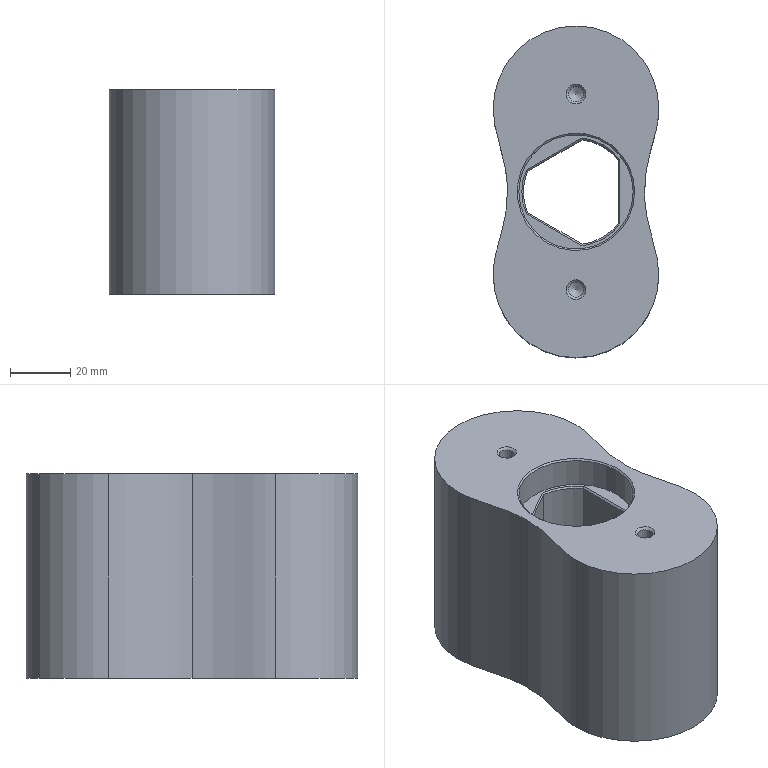NC program | NX | posted with a generic post | part box 55.004 x 110.159 x 68 mm
Lines 28 to 988 of 2889:
(ZLEVEL_PROFILE_COPY_1_COPY , TOOL : D12)
N48 M6
N50 G54
N52 G17 G0 G90 X-3.746 Y8.088 S3000 M3
N54 G43 Z30. H12
N56 Z-2.
N58 G94 G1 X-8.298 Z-2.119 F1000.
N60 X-8.881 Y7.49 Z-2.141
N62 X-10.061 Y5.809 Z-2.195
N64 X-10.927 Y3.946 Z-2.249
N66 X-11.154 Y3.143 Z-2.27
N68 X-2.855 Y-11.231 Z-2.705
N70 X-2.046 Y-11.436 Z-2.727
N72 X0. Y-11.618 Z-2.781
N74 X2.046 Y-11.436 Z-2.835
N76 X2.855 Y-11.231 Z-2.856
N78 X11.154 Y3.143 Z-3.291
N80 X10.927 Y3.946 Z-3.313
N82 X10.061 Y5.809 Z-3.367
N84 X8.881 Y7.49 Z-3.42
N86 X8.298 Y8.088 Z-3.442
N88 X-8.298 Z-3.877
N90 X-8.881 Y7.49 Z-3.899
N92 X-10.061 Y5.809 Z-3.953
N94 X-10.927 Y3.946 Z-4.006
N96 X-11.154 Y3.143 Z-4.028
N98 X-2.855 Y-11.231 Z-4.463
N100 X-2.046 Y-11.436 Z-4.485
N102 X0. Y-11.618 Z-4.538
N104 X2.046 Y-11.436 Z-4.592
N106 X2.855 Y-11.231 Z-4.614
N108 X11.154 Y3.143 Z-5.049
N110 X10.927 Y3.946 Z-5.071
N112 X10.061 Y5.809 Z-5.124
N114 X8.881 Y7.49 Z-5.178
N116 X8.298 Y8.088 Z-5.2
N118 X-8.298 F1800.
N120 G3 X-11.154 Y3.143 R11.588
N122 G1 X-2.855 Y-11.231
N124 G3 X2.855 Y-11.231 R11.588
N126 G1 X11.154 Y3.143
N128 G3 X8.298 Y8.088 R11.588
N130 G1 X-2.75 Y7.895 Z-5.393
N132 X-3.159 Y7.888 Z-5.4
N134 X-8.214
N136 G3 X-10.938 Y3.169 R11.388
N138 G1 X-2.724 Y-11.058
N140 G3 X2.724 Y-11.058 R11.388
N142 G1 X10.938 Y3.169
N144 G3 X8.214 Y7.888 R11.388
N146 G1 X7.804 Y7.882 Z-5.407
N148 X7.395 Y7.877 Z-5.414
N150 X6.986 Y7.872 Z-5.421
N152 X6.577 Y7.868 Z-5.429
N154 X6.168 Y7.864 Z-5.436
N156 X5.759 Y7.861 Z-5.443
N158 X5.349 Y7.859 Z-5.45
N160 X4.94 Y7.856 Z-5.457
N162 X4.531 Y7.854 Z-5.464
N164 X4.122 Y7.853 Z-5.471
N166 X3.712 Y7.852 Z-5.479
N168 X3.303 Y7.851 Z-5.486
N170 X2.894 Y7.85 Z-5.493
N172 X2.485 Z-5.5
N174 X-3.244 Z-5.6
N176 X-8.197
N178 G3 X-10.897 Y3.174 R11.35
N180 G1 X-2.699 Y-11.024
N182 G3 X2.7 Y-11.024 R11.35
N184 G1 X10.897 Y3.174
N186 G3 X8.198 Y7.85 R11.35
N188 G1 X-3.26 Z-5.8
N190 X-8.197
N192 G3 X-10.897 Y3.174 R11.35
N194 G1 X-2.699 Y-11.024
N196 G3 X2.7 Y-11.024 R11.35
N198 G1 X10.897 Y3.174
N200 G3 X8.198 Y7.85 R11.35
N202 G1 X-3.26 Z-6.
N204 X-8.197
N206 G3 X-10.897 Y3.174 R11.35
N208 G1 X-2.699 Y-11.024
N210 G3 X2.7 Y-11.024 R11.35
N212 G1 X10.897 Y3.174
N214 G3 X8.198 Y7.85 R11.35
N216 G1 X-3.26 Z-6.2
N218 X-8.197
N220 G3 X-10.897 Y3.174 R11.35
N222 G1 X-2.699 Y-11.024
N224 G3 X2.7 Y-11.024 R11.35
N226 G1 X10.897 Y3.174
N228 G3 X8.198 Y7.85 R11.35
N230 G1 X-3.26 Z-6.4
N232 X-8.197
N234 G3 X-10.897 Y3.174 R11.35
N236 G1 X-2.699 Y-11.024
N238 G3 X2.7 Y-11.024 R11.35
N240 G1 X10.897 Y3.174
N242 G3 X8.198 Y7.85 R11.35
N244 G1 X-3.26 Z-6.6
N246 X-8.197
N248 G3 X-10.897 Y3.174 R11.35
N250 G1 X-2.699 Y-11.024
N252 G3 X2.7 Y-11.024 R11.35
N254 G1 X10.897 Y3.174
N256 G3 X8.198 Y7.85 R11.35
N258 G1 X-3.26 Z-6.8
N260 X-8.197
N262 G3 X-10.897 Y3.174 R11.35
N264 G1 X-2.699 Y-11.024
N266 G3 X2.7 Y-11.024 R11.35
N268 G1 X10.897 Y3.174
N270 G3 X8.198 Y7.85 R11.35
N272 G1 X-3.26 Z-7.
N274 X-8.197
N276 G3 X-10.897 Y3.174 R11.35
N278 G1 X-2.699 Y-11.024
N280 G3 X2.7 Y-11.024 R11.35
N282 G1 X10.897 Y3.174
N284 G3 X8.198 Y7.85 R11.35
N286 G1 X-3.26 Z-7.2
N288 X-8.197
N290 G3 X-10.897 Y3.174 R11.35
N292 G1 X-2.699 Y-11.024
N294 G3 X2.7 Y-11.024 R11.35
N296 G1 X10.897 Y3.174
N298 G3 X8.198 Y7.85 R11.35
N300 G1 X-3.26 Z-7.4
N302 X-8.197
N304 G3 X-10.897 Y3.174 R11.35
N306 G1 X-2.699 Y-11.024
N308 G3 X2.7 Y-11.024 R11.35
N310 G1 X10.897 Y3.174
N312 G3 X8.198 Y7.85 R11.35
N314 G1 X-3.26 Z-7.6
N316 X-8.197
N318 G3 X-10.897 Y3.174 R11.35
N320 G1 X-2.699 Y-11.024
N322 G3 X2.7 Y-11.024 R11.35
N324 G1 X10.897 Y3.174
N326 G3 X8.198 Y7.85 R11.35
N328 G1 X-3.26 Z-7.8
N330 X-8.197
N332 G3 X-10.897 Y3.174 R11.35
N334 G1 X-2.699 Y-11.024
N336 G3 X2.7 Y-11.024 R11.35
N338 G1 X10.897 Y3.174
N340 G3 X8.198 Y7.85 R11.35
N342 G1 X-3.26 Z-8.
N344 X-8.197
N346 G3 X-10.897 Y3.174 R11.35
N348 G1 X-2.699 Y-11.024
N350 G3 X2.7 Y-11.024 R11.35
N352 G1 X10.897 Y3.174
N354 G3 X8.198 Y7.85 R11.35
N356 G1 X-3.26 Z-8.2
N358 X-8.197
N360 G3 X-10.897 Y3.174 R11.35
N362 G1 X-2.699 Y-11.024
N364 G3 X2.7 Y-11.024 R11.35
N366 G1 X10.897 Y3.174
N368 G3 X8.198 Y7.85 R11.35
N370 G1 X-3.26 Z-8.4
N372 X-8.197
N374 G3 X-10.897 Y3.174 R11.35
N376 G1 X-2.699 Y-11.024
N378 G3 X2.7 Y-11.024 R11.35
N380 G1 X10.897 Y3.174
N382 G3 X8.198 Y7.85 R11.35
N384 G1 X-3.26 Z-8.6
N386 X-8.197
N388 G3 X-10.897 Y3.174 R11.35
N390 G1 X-2.699 Y-11.024
N392 G3 X2.7 Y-11.024 R11.35
N394 G1 X10.897 Y3.174
N396 G3 X8.198 Y7.85 R11.35
N398 G1 X-3.26 Z-8.8
N400 X-8.197
N402 G3 X-10.897 Y3.174 R11.35
N404 G1 X-2.699 Y-11.024
N406 G3 X2.7 Y-11.024 R11.35
N408 G1 X10.897 Y3.174
N410 G3 X8.198 Y7.85 R11.35
N412 G1 X-3.26 Z-9.
N414 X-8.197
N416 G3 X-10.897 Y3.174 R11.35
N418 G1 X-2.699 Y-11.024
N420 G3 X2.7 Y-11.024 R11.35
N422 G1 X10.897 Y3.174
N424 G3 X8.198 Y7.85 R11.35
N426 G1 X-3.26 Z-9.2
N428 X-8.197
N430 G3 X-10.897 Y3.174 R11.35
N432 G1 X-2.699 Y-11.024
N434 G3 X2.7 Y-11.024 R11.35
N436 G1 X10.897 Y3.174
N438 G3 X8.198 Y7.85 R11.35
N440 G1 X-3.26 Z-9.4
N442 X-8.197
N444 G3 X-10.897 Y3.174 R11.35
N446 G1 X-2.699 Y-11.024
N448 G3 X2.7 Y-11.024 R11.35
N450 G1 X10.897 Y3.174
N452 G3 X8.198 Y7.85 R11.35
N454 G1 X-3.26 Z-9.6
N456 X-8.197
N458 G3 X-10.897 Y3.174 R11.35
N460 G1 X-2.699 Y-11.024
N462 G3 X2.7 Y-11.024 R11.35
N464 G1 X10.897 Y3.174
N466 G3 X8.198 Y7.85 R11.35
N468 G1 X-3.26 Z-9.8
N470 X-8.197
N472 G3 X-10.897 Y3.174 R11.35
N474 G1 X-2.699 Y-11.024
N476 G3 X2.7 Y-11.024 R11.35
N478 G1 X10.897 Y3.174
N480 G3 X8.198 Y7.85 R11.35
N482 G1 X-3.26 Z-10.
N484 X-8.197
N486 G3 X-10.897 Y3.174 R11.35
N488 G1 X-2.699 Y-11.024
N490 G3 X2.7 Y-11.024 R11.35
N492 G1 X10.897 Y3.174
N494 G3 X8.198 Y7.85 R11.35
N496 G1 X-3.26 Z-10.2
N498 X-8.197
N500 G3 X-10.897 Y3.174 R11.35
N502 G1 X-2.699 Y-11.024
N504 G3 X2.7 Y-11.024 R11.35
N506 G1 X10.897 Y3.174
N508 G3 X8.198 Y7.85 R11.35
N510 G1 X-3.26 Z-10.4
N512 X-8.197
N514 G3 X-10.897 Y3.174 R11.35
N516 G1 X-2.699 Y-11.024
N518 G3 X2.7 Y-11.024 R11.35
N520 G1 X10.897 Y3.174
N522 G3 X8.198 Y7.85 R11.35
N524 G1 X-3.26 Z-10.6
N526 X-8.197
N528 G3 X-10.897 Y3.174 R11.35
N530 G1 X-2.699 Y-11.024
N532 G3 X2.7 Y-11.024 R11.35
N534 G1 X10.897 Y3.174
N536 G3 X8.198 Y7.85 R11.35
N538 G1 X-3.26 Z-10.8
N540 X-8.197
N542 G3 X-10.897 Y3.174 R11.35
N544 G1 X-2.699 Y-11.024
N546 G3 X2.7 Y-11.024 R11.35
N548 G1 X10.897 Y3.174
N550 G3 X8.198 Y7.85 R11.35
N552 G1 X-3.26 Z-11.
N554 X-8.197
N556 G3 X-10.897 Y3.174 R11.35
N558 G1 X-2.699 Y-11.024
N560 G3 X2.7 Y-11.024 R11.35
N562 G1 X10.897 Y3.174
N564 G3 X8.198 Y7.85 R11.35
N566 G1 X-3.26 Z-11.2
N568 X-8.197
N570 G3 X-10.897 Y3.174 R11.35
N572 G1 X-2.699 Y-11.024
N574 G3 X2.7 Y-11.024 R11.35
N576 G1 X10.897 Y3.174
N578 G3 X8.198 Y7.85 R11.35
N580 G1 X-3.26 Z-11.4
N582 X-8.197
N584 G3 X-10.897 Y3.174 R11.35
N586 G1 X-2.699 Y-11.024
N588 G3 X2.7 Y-11.024 R11.35
N590 G1 X10.897 Y3.174
N592 G3 X8.198 Y7.85 R11.35
N594 G1 X-3.26 Z-11.6
N596 X-8.197
N598 G3 X-10.897 Y3.174 R11.35
N600 G1 X-2.699 Y-11.024
N602 G3 X2.7 Y-11.024 R11.35
N604 G1 X10.897 Y3.174
N606 G3 X8.198 Y7.85 R11.35
N608 G1 X-3.26 Z-11.8
N610 X-8.197
N612 G3 X-10.897 Y3.174 R11.35
N614 G1 X-2.699 Y-11.024
N616 G3 X2.7 Y-11.024 R11.35
N618 G1 X10.897 Y3.174
N620 G3 X8.198 Y7.85 R11.35
N622 G1 X-3.26 Z-12.
N624 X-8.197
N626 G3 X-10.897 Y3.174 R11.35
N628 G1 X-2.699 Y-11.024
N630 G3 X2.7 Y-11.024 R11.35
N632 G1 X10.897 Y3.174
N634 G3 X8.198 Y7.85 R11.35
N636 G1 X-3.26 Z-12.2
N638 X-8.197
N640 G3 X-10.897 Y3.174 R11.35
N642 G1 X-2.699 Y-11.024
N644 G3 X2.7 Y-11.024 R11.35
N646 G1 X10.897 Y3.174
N648 G3 X8.198 Y7.85 R11.35
N650 G1 X-3.26 Z-12.4
N652 X-8.197
N654 G3 X-10.897 Y3.174 R11.35
N656 G1 X-2.699 Y-11.024
N658 G3 X2.7 Y-11.024 R11.35
N660 G1 X10.897 Y3.174
N662 G3 X8.198 Y7.85 R11.35
N664 G1 X-3.26 Z-12.6
N666 X-8.197
N668 G3 X-10.897 Y3.174 R11.35
N670 G1 X-2.699 Y-11.024
N672 G3 X2.7 Y-11.024 R11.35
N674 G1 X10.897 Y3.174
N676 G3 X8.198 Y7.85 R11.35
N678 G1 X-3.26 Z-12.8
N680 X-8.197
N682 G3 X-10.897 Y3.174 R11.35
N684 G1 X-2.699 Y-11.024
N686 G3 X2.7 Y-11.024 R11.35
N688 G1 X10.897 Y3.174
N690 G3 X8.198 Y7.85 R11.35
N692 G1 X-3.26 Z-13.
N694 X-8.197
N696 G3 X-10.897 Y3.174 R11.35
N698 G1 X-2.699 Y-11.024
N700 G3 X2.7 Y-11.024 R11.35
N702 G1 X10.897 Y3.174
N704 G3 X8.198 Y7.85 R11.35
N706 G1 X-3.26 Z-13.2
N708 X-8.197
N710 G3 X-10.897 Y3.174 R11.35
N712 G1 X-2.699 Y-11.024
N714 G3 X2.7 Y-11.024 R11.35
N716 G1 X10.897 Y3.174
N718 G3 X8.198 Y7.85 R11.35
N720 G1 X-3.26 Z-13.4
N722 X-8.197
N724 G3 X-10.897 Y3.174 R11.35
N726 G1 X-2.699 Y-11.024
N728 G3 X2.7 Y-11.024 R11.35
N730 G1 X10.897 Y3.174
N732 G3 X8.198 Y7.85 R11.35
N734 G1 X-3.26 Z-13.6
N736 X-8.197
N738 G3 X-10.897 Y3.174 R11.35
N740 G1 X-2.699 Y-11.024
N742 G3 X2.7 Y-11.024 R11.35
N744 G1 X10.897 Y3.174
N746 G3 X8.198 Y7.85 R11.35
N748 G1 X-3.26 Z-13.8
N750 X-8.197
N752 G3 X-10.897 Y3.174 R11.35
N754 G1 X-2.699 Y-11.024
N756 G3 X2.7 Y-11.024 R11.35
N758 G1 X10.897 Y3.174
N760 G3 X8.198 Y7.85 R11.35
N762 G1 X-3.26 Z-14.
N764 X-8.197
N766 G3 X-10.897 Y3.174 R11.35
N768 G1 X-2.699 Y-11.024
N770 G3 X2.7 Y-11.024 R11.35
N772 G1 X10.897 Y3.174
N774 G3 X8.198 Y7.85 R11.35
N776 G1 X-3.26 Z-14.2
N778 X-8.197
N780 G3 X-10.897 Y3.174 R11.35
N782 G1 X-2.699 Y-11.024
N784 G3 X2.7 Y-11.024 R11.35
N786 G1 X10.897 Y3.174
N788 G3 X8.198 Y7.85 R11.35
N790 G1 X-3.26 Z-14.4
N792 X-8.197
N794 G3 X-10.897 Y3.174 R11.35
N796 G1 X-2.699 Y-11.024
N798 G3 X2.7 Y-11.024 R11.35
N800 G1 X10.897 Y3.174
N802 G3 X8.198 Y7.85 R11.35
N804 G1 X-3.26 Z-14.6
N806 X-8.197
N808 G3 X-10.897 Y3.174 R11.35
N810 G1 X-2.699 Y-11.024
N812 G3 X2.7 Y-11.024 R11.35
N814 G1 X10.897 Y3.174
N816 G3 X8.198 Y7.85 R11.35
N818 G1 X-3.26 Z-14.8
N820 X-8.197
N822 G3 X-10.897 Y3.174 R11.35
N824 G1 X-2.699 Y-11.024
N826 G3 X2.7 Y-11.024 R11.35
N828 G1 X10.897 Y3.174
N830 G3 X8.198 Y7.85 R11.35
N832 G1 X-3.26 Z-15.
N834 X-8.197
N836 G3 X-10.897 Y3.174 R11.35
N838 G1 X-2.699 Y-11.024
N840 G3 X2.7 Y-11.024 R11.35
N842 G1 X10.897 Y3.174
N844 G3 X8.198 Y7.85 R11.35
N846 G1 X-3.26 Z-15.2
N848 X-8.197
N850 G3 X-10.897 Y3.174 R11.35
N852 G1 X-2.699 Y-11.024
N854 G3 X2.7 Y-11.024 R11.35
N856 G1 X10.897 Y3.174
N858 G3 X8.198 Y7.85 R11.35
N860 G1 X-3.26 Z-15.4
N862 X-8.197
N864 G3 X-10.897 Y3.174 R11.35
N866 G1 X-2.699 Y-11.024
N868 G3 X2.7 Y-11.024 R11.35
N870 G1 X10.897 Y3.174
N872 G3 X8.198 Y7.85 R11.35
N874 G1 X-3.26 Z-15.6
N876 X-8.197
N878 G3 X-10.897 Y3.174 R11.35
N880 G1 X-2.699 Y-11.024
N882 G3 X2.7 Y-11.024 R11.35
N884 G1 X10.897 Y3.174
N886 G3 X8.198 Y7.85 R11.35
N888 G1 X-3.26 Z-15.8
N890 X-8.197
N892 G3 X-10.897 Y3.174 R11.35
N894 G1 X-2.699 Y-11.024
N896 G3 X2.7 Y-11.024 R11.35
N898 G1 X10.897 Y3.174
N900 G3 X8.198 Y7.85 R11.35
N902 G1 X-3.26 Z-16.
N904 X-8.197
N906 G3 X-10.897 Y3.174 R11.35
N908 G1 X-2.699 Y-11.024
N910 G3 X2.7 Y-11.024 R11.35
N912 G1 X10.897 Y3.174
N914 G3 X8.198 Y7.85 R11.35
N916 G1 X-3.26 Z-16.2
N918 X-8.197
N920 G3 X-10.897 Y3.174 R11.35
N922 G1 X-2.699 Y-11.024
N924 G3 X2.7 Y-11.024 R11.35
N926 G1 X10.897 Y3.174
N928 G3 X8.198 Y7.85 R11.35
N930 G1 X-3.26 Z-16.4
N932 X-8.197
N934 G3 X-10.897 Y3.174 R11.35
N936 G1 X-2.699 Y-11.024
N938 G3 X2.7 Y-11.024 R11.35
N940 G1 X10.897 Y3.174
N942 G3 X8.198 Y7.85 R11.35
N944 G1 X-3.26 Z-16.6
N946 X-8.197
N948 G3 X-10.897 Y3.174 R11.35
N950 G1 X-2.699 Y-11.024
N952 G3 X2.7 Y-11.024 R11.35
N954 G1 X10.897 Y3.174
N956 G3 X8.198 Y7.85 R11.35
N958 G1 X-3.26 Z-16.8
N960 X-8.197
N962 G3 X-10.897 Y3.174 R11.35
N964 G1 X-2.699 Y-11.024
N966 G3 X2.7 Y-11.024 R11.35
N968 G1 X10.897 Y3.174
N970 G3 X8.198 Y7.85 R11.35
N972 G1 X-3.26 Z-17.
N974 X-8.197
N976 G3 X-10.897 Y3.174 R11.35
N978 G1 X-2.699 Y-11.024
N980 G3 X2.7 Y-11.024 R11.35
N982 G1 X10.897 Y3.174
N984 G3 X8.198 Y7.85 R11.35
N986 G1 X-3.26 Z-17.2
N988 X-8.197
N990 G3 X-10.897 Y3.174 R11.35
N992 G1 X-2.699 Y-11.024
N994 G3 X2.7 Y-11.024 R11.35
N996 G1 X10.897 Y3.174
N998 G3 X8.198 Y7.85 R11.35
N1000 G1 X-3.26 Z-17.4
N1002 X-8.197
N1004 G3 X-10.897 Y3.174 R11.35
N1006 G1 X-2.699 Y-11.024
N1008 G3 X2.7 Y-11.024 R11.35
N1010 G1 X10.897 Y3.174
N1012 G3 X8.198 Y7.85 R11.35
N1014 G1 X-3.26 Z-17.6
N1016 X-8.197
N1018 G3 X-10.897 Y3.174 R11.35
N1020 G1 X-2.699 Y-11.024
N1022 G3 X2.7 Y-11.024 R11.35
N1024 G1 X10.897 Y3.174
N1026 G3 X8.198 Y7.85 R11.35
N1028 G1 X-3.26 Z-17.8
N1030 X-8.197
N1032 G3 X-10.897 Y3.174 R11.35
N1034 G1 X-2.699 Y-11.024
N1036 G3 X2.7 Y-11.024 R11.35
N1038 G1 X10.897 Y3.174
N1040 G3 X8.198 Y7.85 R11.35
N1042 G1 X-3.26 Z-18.
N1044 X-8.197
N1046 G3 X-10.897 Y3.174 R11.35
N1048 G1 X-2.699 Y-11.024
N1050 G3 X2.7 Y-11.024 R11.35
N1052 G1 X10.897 Y3.174
N1054 G3 X8.198 Y7.85 R11.35
N1056 G1 X-3.26 Z-18.2
N1058 X-8.197
N1060 G3 X-10.897 Y3.174 R11.35
N1062 G1 X-2.699 Y-11.024
N1064 G3 X2.7 Y-11.024 R11.35
N1066 G1 X10.897 Y3.174
N1068 G3 X8.198 Y7.85 R11.35
N1070 G1 X-3.26 Z-18.4
N1072 X-8.197
N1074 G3 X-10.897 Y3.174 R11.35
N1076 G1 X-2.699 Y-11.024
N1078 G3 X2.7 Y-11.024 R11.35
N1080 G1 X10.897 Y3.174
N1082 G3 X8.198 Y7.85 R11.35
N1084 G1 X-3.26 Z-18.6
N1086 X-8.197
N1088 G3 X-10.897 Y3.174 R11.35
N1090 G1 X-2.699 Y-11.024
N1092 G3 X2.7 Y-11.024 R11.35
N1094 G1 X10.897 Y3.174
N1096 G3 X8.198 Y7.85 R11.35
N1098 G1 X-3.26 Z-18.8
N1100 X-8.197
N1102 G3 X-10.897 Y3.174 R11.35
N1104 G1 X-2.699 Y-11.024
N1106 G3 X2.7 Y-11.024 R11.35
N1108 G1 X10.897 Y3.174
N1110 G3 X8.198 Y7.85 R11.35
N1112 G1 X-3.26 Z-19.
N1114 X-8.197
N1116 G3 X-10.897 Y3.174 R11.35
N1118 G1 X-2.699 Y-11.024
N1120 G3 X2.7 Y-11.024 R11.35
N1122 G1 X10.897 Y3.174
N1124 G3 X8.198 Y7.85 R11.35
N1126 G1 X-3.26 Z-19.2
N1128 X-8.197
N1130 G3 X-10.897 Y3.174 R11.35
N1132 G1 X-2.699 Y-11.024
N1134 G3 X2.7 Y-11.024 R11.35
N1136 G1 X10.897 Y3.174
N1138 G3 X8.198 Y7.85 R11.35
N1140 G1 X-3.26 Z-19.4
N1142 X-8.197
N1144 G3 X-10.897 Y3.174 R11.35
N1146 G1 X-2.699 Y-11.024
N1148 G3 X2.7 Y-11.024 R11.35
N1150 G1 X10.897 Y3.174
N1152 G3 X8.198 Y7.85 R11.35
N1154 G1 X-3.26 Z-19.6
N1156 X-8.197
N1158 G3 X-10.897 Y3.174 R11.35
N1160 G1 X-2.699 Y-11.024
N1162 G3 X2.7 Y-11.024 R11.35
N1164 G1 X10.897 Y3.174
N1166 G3 X8.198 Y7.85 R11.35
N1168 G1 X-3.26 Z-19.8
N1170 X-8.197
N1172 G3 X-10.897 Y3.174 R11.35
N1174 G1 X-2.699 Y-11.024
N1176 G3 X2.7 Y-11.024 R11.35
N1178 G1 X10.897 Y3.174
N1180 G3 X8.198 Y7.85 R11.35
N1182 G1 X-3.26 Z-20.
N1184 X-8.197
N1186 G3 X-10.897 Y3.174 R11.35
N1188 G1 X-2.699 Y-11.024
N1190 G3 X2.7 Y-11.024 R11.35
N1192 G1 X10.897 Y3.174
N1194 G3 X8.198 Y7.85 R11.35
N1196 G1 X-3.26 Z-20.2
N1198 X-8.197
N1200 G3 X-10.897 Y3.174 R11.35
N1202 G1 X-2.699 Y-11.024
N1204 G3 X2.7 Y-11.024 R11.35
N1206 G1 X10.897 Y3.174
N1208 G3 X8.198 Y7.85 R11.35
N1210 G1 X-3.26 Z-20.4
N1212 X-8.197
N1214 G3 X-10.897 Y3.174 R11.35
N1216 G1 X-2.699 Y-11.024
N1218 G3 X2.7 Y-11.024 R11.35
N1220 G1 X10.897 Y3.174
N1222 G3 X8.198 Y7.85 R11.35
N1224 G1 X-3.26 Z-20.6
N1226 X-8.197
N1228 G3 X-10.897 Y3.174 R11.35
N1230 G1 X-2.699 Y-11.024
N1232 G3 X2.7 Y-11.024 R11.35
N1234 G1 X10.897 Y3.174
N1236 G3 X8.198 Y7.85 R11.35
N1238 G1 X-3.26 Z-20.8
N1240 X-8.197
N1242 G3 X-10.897 Y3.174 R11.35
N1244 G1 X-2.699 Y-11.024
N1246 G3 X2.7 Y-11.024 R11.35
N1248 G1 X10.897 Y3.174
N1250 G3 X8.198 Y7.85 R11.35
N1252 G1 X-3.26 Z-21.
N1254 X-8.197
N1256 G3 X-10.897 Y3.174 R11.35
N1258 G1 X-2.699 Y-11.024
N1260 G3 X2.7 Y-11.024 R11.35
N1262 G1 X10.897 Y3.174
N1264 G3 X8.198 Y7.85 R11.35
N1266 G1 X-3.26 Z-21.2
N1268 X-8.197
N1270 G3 X-10.897 Y3.174 R11.35
N1272 G1 X-2.699 Y-11.024
N1274 G3 X2.7 Y-11.024 R11.35
N1276 G1 X10.897 Y3.174
N1278 G3 X8.198 Y7.85 R11.35
N1280 G1 X-3.26 Z-21.4
N1282 X-8.197
N1284 G3 X-10.897 Y3.174 R11.35
N1286 G1 X-2.699 Y-11.024
N1288 G3 X2.7 Y-11.024 R11.35
N1290 G1 X10.897 Y3.174
N1292 G3 X8.198 Y7.85 R11.35
N1294 G1 X-3.26 Z-21.6
N1296 X-8.197
N1298 G3 X-10.897 Y3.174 R11.35
N1300 G1 X-2.699 Y-11.024
N1302 G3 X2.7 Y-11.024 R11.35
N1304 G1 X10.897 Y3.174
N1306 G3 X8.198 Y7.85 R11.35
N1308 G1 X-3.26 Z-21.8
N1310 X-8.197
N1312 G3 X-10.897 Y3.174 R11.35
N1314 G1 X-2.699 Y-11.024
N1316 G3 X2.7 Y-11.024 R11.35
N1318 G1 X10.897 Y3.174
N1320 G3 X8.198 Y7.85 R11.35
N1322 G1 X-3.26 Z-22.
N1324 X-8.197
N1326 G3 X-10.897 Y3.174 R11.35
N1328 G1 X-2.699 Y-11.024
N1330 G3 X2.7 Y-11.024 R11.35
N1332 G1 X10.897 Y3.174
N1334 G3 X8.198 Y7.85 R11.35
N1336 G1 X-3.26 Z-22.2
N1338 X-8.197
N1340 G3 X-10.897 Y3.174 R11.35
N1342 G1 X-2.699 Y-11.024
N1344 G3 X2.7 Y-11.024 R11.35
N1346 G1 X10.897 Y3.174
N1348 G3 X8.198 Y7.85 R11.35
N1350 G1 X-3.26 Z-22.4
N1352 X-8.197
N1354 G3 X-10.897 Y3.174 R11.35
N1356 G1 X-2.699 Y-11.024
N1358 G3 X2.7 Y-11.024 R11.35
N1360 G1 X10.897 Y3.174
N1362 G3 X8.198 Y7.85 R11.35
N1364 G1 X-3.26 Z-22.6
N1366 X-8.197
N1368 G3 X-10.897 Y3.174 R11.35
N1370 G1 X-2.699 Y-11.024
N1372 G3 X2.7 Y-11.024 R11.35
N1374 G1 X10.897 Y3.174
N1376 G3 X8.198 Y7.85 R11.35
N1378 G1 X-3.26 Z-22.8
N1380 X-8.197
N1382 G3 X-10.897 Y3.174 R11.35
N1384 G1 X-2.699 Y-11.024
N1386 G3 X2.7 Y-11.024 R11.35
N1388 G1 X10.897 Y3.174
N1390 G3 X8.198 Y7.85 R11.35
N1392 G1 X-3.26 Z-23.
N1394 X-8.197
N1396 G3 X-10.897 Y3.174 R11.35
N1398 G1 X-2.699 Y-11.024
N1400 G3 X2.7 Y-11.024 R11.35
N1402 G1 X10.897 Y3.174
N1404 G3 X8.198 Y7.85 R11.35
N1406 G1 X-3.26 Z-23.2
N1408 X-8.197
N1410 G3 X-10.897 Y3.174 R11.35
N1412 G1 X-2.699 Y-11.024
N1414 G3 X2.7 Y-11.024 R11.35
N1416 G1 X10.897 Y3.174
N1418 G3 X8.198 Y7.85 R11.35
N1420 G1 X-3.26 Z-23.4
N1422 X-8.197
N1424 G3 X-10.897 Y3.174 R11.35
N1426 G1 X-2.699 Y-11.024
N1428 G3 X2.7 Y-11.024 R11.35
N1430 G1 X10.897 Y3.174
N1432 G3 X8.198 Y7.85 R11.35
N1434 G1 X-3.26 Z-23.6
N1436 X-8.197
N1438 G3 X-10.897 Y3.174 R11.35
N1440 G1 X-2.699 Y-11.024
N1442 G3 X2.7 Y-11.024 R11.35
N1444 G1 X10.897 Y3.174
N1446 G3 X8.198 Y7.85 R11.35
N1448 G1 X-3.26 Z-23.8
N1450 X-8.197
N1452 G3 X-10.897 Y3.174 R11.35
N1454 G1 X-2.699 Y-11.024
N1456 G3 X2.7 Y-11.024 R11.35
N1458 G1 X10.897 Y3.174
N1460 G3 X8.198 Y7.85 R11.35
N1462 G1 X-3.26 Z-24.
N1464 X-8.197
N1466 G3 X-10.897 Y3.174 R11.35
N1468 G1 X-2.699 Y-11.024
N1470 G3 X2.7 Y-11.024 R11.35
N1472 G1 X10.897 Y3.174
N1474 G3 X8.198 Y7.85 R11.35
N1476 G1 X-3.26 Z-24.2
N1478 X-8.197
N1480 G3 X-10.897 Y3.174 R11.35
N1482 G1 X-2.699 Y-11.024
N1484 G3 X2.7 Y-11.024 R11.35
N1486 G1 X10.897 Y3.174
N1488 G3 X8.198 Y7.85 R11.35
N1490 G1 X-3.26 Z-24.4
N1492 X-8.197
N1494 G3 X-10.897 Y3.174 R11.35
N1496 G1 X-2.699 Y-11.024
N1498 G3 X2.7 Y-11.024 R11.35
N1500 G1 X10.897 Y3.174
N1502 G3 X8.198 Y7.85 R11.35
N1504 G1 X-3.26 Z-24.6
N1506 X-8.197
N1508 G3 X-10.897 Y3.174 R11.35
N1510 G1 X-2.699 Y-11.024
N1512 G3 X2.7 Y-11.024 R11.35
N1514 G1 X10.897 Y3.174
N1516 G3 X8.198 Y7.85 R11.35
N1518 G1 X-3.26 Z-24.8
N1520 X-8.197
N1522 G3 X-10.897 Y3.174 R11.35
N1524 G1 X-2.699 Y-11.024
N1526 G3 X2.7 Y-11.024 R11.35
N1528 G1 X10.897 Y3.174
N1530 G3 X8.198 Y7.85 R11.35
N1532 G1 X-3.26 Z-25.
N1534 X-8.197
N1536 G3 X-10.897 Y3.174 R11.35
N1538 G1 X-2.699 Y-11.024
N1540 G3 X2.7 Y-11.024 R11.35
N1542 G1 X10.897 Y3.174
N1544 G3 X8.198 Y7.85 R11.35
N1546 G1 X-3.26 Z-25.2
N1548 X-8.197
N1550 G3 X-10.897 Y3.174 R11.35
N1552 G1 X-2.699 Y-11.024
N1554 G3 X2.7 Y-11.024 R11.35
N1556 G1 X10.897 Y3.174
N1558 G3 X8.198 Y7.85 R11.35
N1560 G1 X-3.26 Z-25.4
N1562 X-8.197
N1564 G3 X-10.897 Y3.174 R11.35
N1566 G1 X-2.699 Y-11.024
N1568 G3 X2.7 Y-11.024 R11.35
N1570 G1 X10.897 Y3.174
N1572 G3 X8.198 Y7.85 R11.35
N1574 G1 X-3.26 Z-25.6
N1576 X-8.197
N1578 G3 X-10.897 Y3.174 R11.35
N1580 G1 X-2.699 Y-11.024
N1582 G3 X2.7 Y-11.024 R11.35
N1584 G1 X10.897 Y3.174
N1586 G3 X8.198 Y7.85 R11.35
N1588 G1 X-3.26 Z-25.8
N1590 X-8.197
N1592 G3 X-10.897 Y3.174 R11.35
N1594 G1 X-2.699 Y-11.024
N1596 G3 X2.7 Y-11.024 R11.35
N1598 G1 X10.897 Y3.174
N1600 G3 X8.198 Y7.85 R11.35
N1602 G1 X-3.26 Z-26.
N1604 X-8.197
N1606 G3 X-10.897 Y3.174 R11.35
N1608 G1 X-2.699 Y-11.024
N1610 G3 X2.7 Y-11.024 R11.35
N1612 G1 X10.897 Y3.174
N1614 G3 X8.198 Y7.85 R11.35
N1616 G1 X-3.26 Z-26.2
N1618 X-8.197
N1620 G3 X-10.897 Y3.174 R11.35
N1622 G1 X-2.699 Y-11.024
N1624 G3 X2.7 Y-11.024 R11.35
N1626 G1 X10.897 Y3.174
N1628 G3 X8.198 Y7.85 R11.35
N1630 G1 X-3.26 Z-26.4
N1632 X-8.197
N1634 G3 X-10.897 Y3.174 R11.35
N1636 G1 X-2.699 Y-11.024
N1638 G3 X2.7 Y-11.024 R11.35
N1640 G1 X10.897 Y3.174
N1642 G3 X8.198 Y7.85 R11.35
N1644 G1 X-3.26 Z-26.6
N1646 X-8.197
N1648 G3 X-10.897 Y3.174 R11.35
N1650 G1 X-2.699 Y-11.024
N1652 G3 X2.7 Y-11.024 R11.35
N1654 G1 X10.897 Y3.174
N1656 G3 X8.198 Y7.85 R11.35
N1658 G1 X-3.26 Z-26.8
N1660 X-8.197
N1662 G3 X-10.897 Y3.174 R11.35
N1664 G1 X-2.699 Y-11.024
N1666 G3 X2.7 Y-11.024 R11.35
N1668 G1 X10.897 Y3.174
N1670 G3 X8.198 Y7.85 R11.35
N1672 G1 X-3.26 Z-27.
N1674 X-8.197
N1676 G3 X-10.897 Y3.174 R11.35
N1678 G1 X-2.699 Y-11.024
N1680 G3 X2.7 Y-11.024 R11.35
N1682 G1 X10.897 Y3.174
N1684 G3 X8.198 Y7.85 R11.35
N1686 G1 X-3.26 Z-27.2
N1688 X-8.197
N1690 G3 X-10.897 Y3.174 R11.35
N1692 G1 X-2.699 Y-11.024
N1694 G3 X2.7 Y-11.024 R11.35
N1696 G1 X10.897 Y3.174
N1698 G3 X8.198 Y7.85 R11.35
N1700 G1 X-3.26 Z-27.4
N1702 X-8.197
N1704 G3 X-10.897 Y3.174 R11.35
N1706 G1 X-2.699 Y-11.024
N1708 G3 X2.7 Y-11.024 R11.35
N1710 G1 X10.897 Y3.174
N1712 G3 X8.198 Y7.85 R11.35
N1714 G1 X-3.26 Z-27.6
N1716 X-8.197
N1718 G3 X-10.897 Y3.174 R11.35
N1720 G1 X-2.699 Y-11.024
N1722 G3 X2.7 Y-11.024 R11.35
N1724 G1 X10.897 Y3.174
N1726 G3 X8.198 Y7.85 R11.35
N1728 G1 X-3.26 Z-27.8
N1730 X-8.197
N1732 G3 X-10.897 Y3.174 R11.35
N1734 G1 X-2.699 Y-11.024
N1736 G3 X2.7 Y-11.024 R11.35
N1738 G1 X10.897 Y3.174
N1740 G3 X8.198 Y7.85 R11.35
N1742 G1 X-3.26 Z-28.
N1744 X-8.197
N1746 G3 X-10.897 Y3.174 R11.35
N1748 G1 X-2.699 Y-11.024
N1750 G3 X2.7 Y-11.024 R11.35
N1752 G1 X10.897 Y3.174
N1754 G3 X8.198 Y7.85 R11.35
N1756 G1 X-3.26 Z-28.2
N1758 X-8.197
N1760 G3 X-10.897 Y3.174 R11.35
N1762 G1 X-2.699 Y-11.024
N1764 G3 X2.7 Y-11.024 R11.35
N1766 G1 X10.897 Y3.174
N1768 G3 X8.198 Y7.85 R11.35
N1770 G1 X-3.26 Z-28.4
N1772 X-8.197
N1774 G3 X-10.897 Y3.174 R11.35
N1776 G1 X-2.699 Y-11.024
N1778 G3 X2.7 Y-11.024 R11.35
N1780 G1 X10.897 Y3.174
N1782 G3 X8.198 Y7.85 R11.35
N1784 G1 X-3.26 Z-28.6
N1786 X-8.197
N1788 G3 X-10.897 Y3.174 R11.35
N1790 G1 X-2.699 Y-11.024
N1792 G3 X2.7 Y-11.024 R11.35
N1794 G1 X10.897 Y3.174
N1796 G3 X8.198 Y7.85 R11.35
N1798 G1 X-3.26 Z-28.8
N1800 X-8.197
N1802 G3 X-10.897 Y3.174 R11.35
N1804 G1 X-2.699 Y-11.024
N1806 G3 X2.7 Y-11.024 R11.35
N1808 G1 X10.897 Y3.174
N1810 G3 X8.198 Y7.85 R11.35
N1812 G1 X-3.26 Z-29.
N1814 X-8.197
N1816 G3 X-10.897 Y3.174 R11.35
N1818 G1 X-2.699 Y-11.024
N1820 G3 X2.7 Y-11.024 R11.35
N1822 G1 X10.897 Y3.174
N1824 G3 X8.198 Y7.85 R11.35
N1826 G1 X-3.26 Z-29.2
N1828 X-8.197
N1830 G3 X-10.897 Y3.174 R11.35
N1832 G1 X-2.699 Y-11.024
N1834 G3 X2.7 Y-11.024 R11.35
N1836 G1 X10.897 Y3.174
N1838 G3 X8.198 Y7.85 R11.35
N1840 G1 X-3.26 Z-29.4
N1842 X-8.197
N1844 G3 X-10.897 Y3.174 R11.35
N1846 G1 X-2.699 Y-11.024
N1848 G3 X2.7 Y-11.024 R11.35
N1850 G1 X10.897 Y3.174
N1852 G3 X8.198 Y7.85 R11.35
N1854 G1 X-3.26 Z-29.6
N1856 X-8.197
N1858 G3 X-10.897 Y3.174 R11.35
N1860 G1 X-2.699 Y-11.024
N1862 G3 X2.7 Y-11.024 R11.35
N1864 G1 X10.897 Y3.174
N1866 G3 X8.198 Y7.85 R11.35
N1868 G1 X-3.26 Z-29.8
N1870 X-8.197
N1872 G3 X-10.897 Y3.174 R11.35
N1874 G1 X-2.699 Y-11.024
N1876 G3 X2.7 Y-11.024 R11.35
N1878 G1 X10.897 Y3.174
N1880 G3 X8.198 Y7.85 R11.35
N1882 G1 X-3.26 Z-30.
N1884 X-8.197
N1886 G3 X-10.897 Y3.174 R11.35
N1888 G1 X-2.699 Y-11.024
N1890 G3 X2.7 Y-11.024 R11.35
N1892 G1 X10.897 Y3.174
N1894 G3 X8.198 Y7.85 R11.35
N1896 G1 X-3.26 Z-30.2
N1898 X-8.197
N1900 G3 X-10.897 Y3.174 R11.35
N1902 G1 X-2.699 Y-11.024
N1904 G3 X2.7 Y-11.024 R11.35
N1906 G1 X10.897 Y3.174
N1908 G3 X8.198 Y7.85 R11.35
N1910 G1 X-3.26 Z-30.4
N1912 X-8.197
N1914 G3 X-10.897 Y3.174 R11.35
N1916 G1 X-2.699 Y-11.024
N1918 G3 X2.7 Y-11.024 R11.35
N1920 G1 X10.897 Y3.174
N1922 G3 X8.198 Y7.85 R11.35
N1924 G1 X-3.26 Z-30.6
N1926 X-8.197
N1928 G3 X-10.897 Y3.174 R11.35
N1930 G1 X-2.699 Y-11.024
N1932 G3 X2.7 Y-11.024 R11.35
N1934 G1 X10.897 Y3.174
N1936 G3 X8.198 Y7.85 R11.35
N1938 G1 X-3.26 Z-30.8
N1940 X-8.197
N1942 G3 X-10.897 Y3.174 R11.35
N1944 G1 X-2.699 Y-11.024
N1946 G3 X2.7 Y-11.024 R11.35
N1948 G1 X10.897 Y3.174
N1950 G3 X8.198 Y7.85 R11.35
N1952 G1 X-3.26 Z-31.
N1954 X-8.197
N1956 G3 X-10.897 Y3.174 R11.35
N1958 G1 X-2.699 Y-11.024
N1960 G3 X2.7 Y-11.024 R11.35
N1962 G1 X10.897 Y3.174